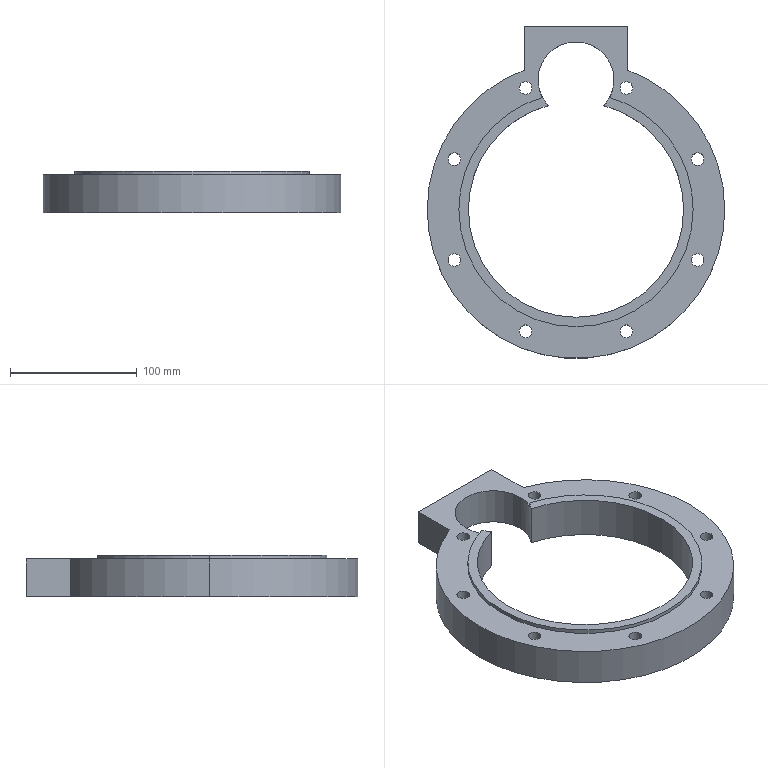Part | SolidWorks | features ICE 2, Cut 1, Extrusion 1, HoleWzd 1 | 1 solid | 34 faces | box 235 x 262.5 x 33 mm | volume 612977 mm3 | cylinder 28 | plane 6 | commonest cylinder face diameters 10 x16 60 x3 170 x3 185 x3 235 x3
STEP:
#1=CARTESIAN_POINT('',(26.584,88.598,30.));
#2=VERTEX_POINT('',#1);
#3=CARTESIAN_POINT('',(30.,102.5,30.));
#4=VERTEX_POINT('',#3);
#5=CARTESIAN_POINT('',(0.,102.5,30.));
#6=DIRECTION('',(0.,0.,1.));
#7=DIRECTION('',(1.,0.,0.));
#8=AXIS2_PLACEMENT_3D('',#5,#6,#7);
#9=CIRCLE('',#8,30.);
#10=EDGE_CURVE('',#2,#4,#9,.T.);
#11=ORIENTED_EDGE('',*,*,#10,.T.);
#12=CARTESIAN_POINT('',(30.,102.5,0.));
#13=VERTEX_POINT('',#12);
#14=CARTESIAN_POINT('',(30.,102.5,33.));
#15=DIRECTION('',(0.,0.,-1.));
#16=VECTOR('',#15,1000.);
#17=LINE('',#14,#16);
#18=EDGE_CURVE('',#4,#13,#17,.T.);
#19=ORIENTED_EDGE('',*,*,#18,.T.);
#20=CARTESIAN_POINT('',(22.,82.104,0.));
#21=VERTEX_POINT('',#20);
#22=CARTESIAN_POINT('',(0.,102.5,0.));
#23=DIRECTION('',(0.,0.,-1.));
#24=DIRECTION('',(-1.,0.,0.));
#25=AXIS2_PLACEMENT_3D('',#22,#23,#24);
#26=CIRCLE('',#25,30.);
#27=EDGE_CURVE('',#13,#21,#26,.T.);
#28=ORIENTED_EDGE('',*,*,#27,.T.);
#29=CARTESIAN_POINT('',(22.,82.104,33.));
#30=VERTEX_POINT('',#29);
#31=CARTESIAN_POINT('',(22.,82.104,16.5));
#32=DIRECTION('',(0.,0.,1.));
#33=VECTOR('',#32,1000.);
#34=LINE('',#31,#33);
#35=EDGE_CURVE('',#21,#30,#34,.T.);
#36=ORIENTED_EDGE('',*,*,#35,.T.);
#37=CARTESIAN_POINT('',(26.584,88.598,33.));
#38=VERTEX_POINT('',#37);
#39=CARTESIAN_POINT('',(0.,102.5,33.));
#40=DIRECTION('',(0.,0.,-1.));
#41=DIRECTION('',(-1.,0.,0.));
#42=AXIS2_PLACEMENT_3D('',#39,#40,#41);
#43=CIRCLE('',#42,30.);
#44=EDGE_CURVE('',#38,#30,#43,.T.);
#45=ORIENTED_EDGE('',*,*,#44,.F.);
#46=CARTESIAN_POINT('',(26.584,88.598,16.5));
#47=DIRECTION('',(0.,0.,1.));
#48=VECTOR('',#47,1000.);
#49=LINE('',#46,#48);
#50=EDGE_CURVE('',#2,#38,#49,.T.);
#51=ORIENTED_EDGE('',*,*,#50,.F.);
#52=EDGE_LOOP('',(#11,#19,#28,#36,#45,#51));
#53=FACE_OUTER_BOUND('',#52,.T.);
#54=CARTESIAN_POINT('',(0.,102.5,33.));
#55=DIRECTION('',(0.,0.,-1.));
#56=DIRECTION('',(-1.,0.,0.));
#57=AXIS2_PLACEMENT_3D('',#54,#55,#56);
#58=CYLINDRICAL_SURFACE('',#57,30.);
#59=ADVANCED_FACE('',(#53),#58,.F.);
#60=ORIENTED_EDGE('',*,*,#18,.F.);
#61=CARTESIAN_POINT('',(-30.,102.5,30.));
#62=VERTEX_POINT('',#61);
#63=CARTESIAN_POINT('',(0.,102.5,30.));
#64=DIRECTION('',(0.,0.,1.));
#65=DIRECTION('',(1.,0.,0.));
#66=AXIS2_PLACEMENT_3D('',#63,#64,#65);
#67=CIRCLE('',#66,30.);
#68=EDGE_CURVE('',#4,#62,#67,.T.);
#69=ORIENTED_EDGE('',*,*,#68,.T.);
#70=CARTESIAN_POINT('',(-30.,102.5,0.));
#71=VERTEX_POINT('',#70);
#72=CARTESIAN_POINT('',(-30.,102.5,33.));
#73=DIRECTION('',(0.,0.,-1.));
#74=VECTOR('',#73,1000.);
#75=LINE('',#72,#74);
#76=EDGE_CURVE('',#62,#71,#75,.T.);
#77=ORIENTED_EDGE('',*,*,#76,.T.);
#78=CARTESIAN_POINT('',(0.,102.5,0.));
#79=DIRECTION('',(0.,0.,-1.));
#80=DIRECTION('',(-1.,0.,0.));
#81=AXIS2_PLACEMENT_3D('',#78,#79,#80);
#82=CIRCLE('',#81,30.);
#83=EDGE_CURVE('',#71,#13,#82,.T.);
#84=ORIENTED_EDGE('',*,*,#83,.T.);
#85=EDGE_LOOP('',(#60,#69,#77,#84));
#86=FACE_OUTER_BOUND('',#85,.T.);
#87=CARTESIAN_POINT('',(0.,102.5,33.));
#88=DIRECTION('',(0.,0.,-1.));
#89=DIRECTION('',(-1.,0.,0.));
#90=AXIS2_PLACEMENT_3D('',#87,#88,#89);
#91=CYLINDRICAL_SURFACE('',#90,30.);
#92=ADVANCED_FACE('',(#86),#91,.F.);
#93=CARTESIAN_POINT('',(92.5,0.,33.));
#94=VERTEX_POINT('',#93);
#95=CARTESIAN_POINT('',(0.,0.,33.));
#96=DIRECTION('',(0.,0.,1.));
#97=DIRECTION('',(1.,0.,0.));
#98=AXIS2_PLACEMENT_3D('',#95,#96,#97);
#99=CIRCLE('',#98,92.5);
#100=EDGE_CURVE('',#94,#38,#99,.T.);
#101=ORIENTED_EDGE('',*,*,#100,.F.);
#102=CARTESIAN_POINT('',(92.5,0.,30.));
#103=VERTEX_POINT('',#102);
#104=CARTESIAN_POINT('',(92.5,0.,33.));
#105=DIRECTION('',(0.,0.,-1.));
#106=VECTOR('',#105,1000.);
#107=LINE('',#104,#106);
#108=EDGE_CURVE('',#94,#103,#107,.T.);
#109=ORIENTED_EDGE('',*,*,#108,.T.);
#110=CARTESIAN_POINT('',(0.,0.,30.));
#111=DIRECTION('',(0.,0.,1.));
#112=DIRECTION('',(1.,0.,0.));
#113=AXIS2_PLACEMENT_3D('',#110,#111,#112);
#114=CIRCLE('',#113,92.5);
#115=EDGE_CURVE('',#103,#2,#114,.T.);
#116=ORIENTED_EDGE('',*,*,#115,.T.);
#117=ORIENTED_EDGE('',*,*,#50,.T.);
#118=EDGE_LOOP('',(#101,#109,#116,#117));
#119=FACE_OUTER_BOUND('',#118,.T.);
#120=CARTESIAN_POINT('',(0.,0.,33.));
#121=DIRECTION('',(0.,0.,-1.));
#122=DIRECTION('',(-1.,0.,0.));
#123=AXIS2_PLACEMENT_3D('',#120,#121,#122);
#124=CYLINDRICAL_SURFACE('',#123,92.5);
#125=ADVANCED_FACE('',(#119),#124,.T.);
#126=ORIENTED_EDGE('',*,*,#108,.F.);
#127=CARTESIAN_POINT('',(-92.5,0.,33.));
#128=VERTEX_POINT('',#127);
#129=CARTESIAN_POINT('',(0.,0.,33.));
#130=DIRECTION('',(0.,0.,1.));
#131=DIRECTION('',(1.,0.,0.));
#132=AXIS2_PLACEMENT_3D('',#129,#130,#131);
#133=CIRCLE('',#132,92.5);
#134=EDGE_CURVE('',#128,#94,#133,.T.);
#135=ORIENTED_EDGE('',*,*,#134,.F.);
#136=CARTESIAN_POINT('',(-92.5,0.,30.));
#137=VERTEX_POINT('',#136);
#138=CARTESIAN_POINT('',(-92.5,0.,33.));
#139=DIRECTION('',(0.,0.,-1.));
#140=VECTOR('',#139,1000.);
#141=LINE('',#138,#140);
#142=EDGE_CURVE('',#128,#137,#141,.T.);
#143=ORIENTED_EDGE('',*,*,#142,.T.);
#144=CARTESIAN_POINT('',(0.,0.,30.));
#145=DIRECTION('',(0.,0.,1.));
#146=DIRECTION('',(1.,0.,0.));
#147=AXIS2_PLACEMENT_3D('',#144,#145,#146);
#148=CIRCLE('',#147,92.5);
#149=EDGE_CURVE('',#137,#103,#148,.T.);
#150=ORIENTED_EDGE('',*,*,#149,.T.);
#151=EDGE_LOOP('',(#126,#135,#143,#150));
#152=FACE_OUTER_BOUND('',#151,.T.);
#153=CARTESIAN_POINT('',(0.,0.,33.));
#154=DIRECTION('',(0.,0.,-1.));
#155=DIRECTION('',(-1.,0.,0.));
#156=AXIS2_PLACEMENT_3D('',#153,#154,#155);
#157=CYLINDRICAL_SURFACE('',#156,92.5);
#158=ADVANCED_FACE('',(#152),#157,.T.);
#159=CARTESIAN_POINT('',(44.799,96.083,30.));
#160=VERTEX_POINT('',#159);
#161=CARTESIAN_POINT('',(34.799,96.083,30.));
#162=VERTEX_POINT('',#161);
#163=CARTESIAN_POINT('',(39.799,96.083,30.));
#164=DIRECTION('',(0.,0.,-1.));
#165=DIRECTION('',(-1.,0.,0.));
#166=AXIS2_PLACEMENT_3D('',#163,#164,#165);
#167=CIRCLE('',#166,5.);
#168=EDGE_CURVE('',#160,#162,#167,.T.);
#169=ORIENTED_EDGE('',*,*,#168,.F.);
#170=CARTESIAN_POINT('',(44.799,96.083,0.));
#171=VERTEX_POINT('',#170);
#172=CARTESIAN_POINT('',(44.799,96.083,0.));
#173=DIRECTION('',(0.,0.,-1.));
#174=VECTOR('',#173,1000.);
#175=LINE('',#172,#174);
#176=EDGE_CURVE('',#160,#171,#175,.T.);
#177=ORIENTED_EDGE('',*,*,#176,.T.);
#178=CARTESIAN_POINT('',(34.799,96.083,0.));
#179=VERTEX_POINT('',#178);
#180=CARTESIAN_POINT('',(39.799,96.083,0.));
#181=DIRECTION('',(0.,0.,-1.));
#182=DIRECTION('',(-1.,0.,0.));
#183=AXIS2_PLACEMENT_3D('',#180,#181,#182);
#184=CIRCLE('',#183,5.);
#185=EDGE_CURVE('',#171,#179,#184,.T.);
#186=ORIENTED_EDGE('',*,*,#185,.T.);
#187=CARTESIAN_POINT('',(34.799,96.083,0.));
#188=DIRECTION('',(0.,0.,-1.));
#189=VECTOR('',#188,1000.);
#190=LINE('',#187,#189);
#191=EDGE_CURVE('',#162,#179,#190,.T.);
#192=ORIENTED_EDGE('',*,*,#191,.F.);
#193=EDGE_LOOP('',(#169,#177,#186,#192));
#194=FACE_OUTER_BOUND('',#193,.T.);
#195=CARTESIAN_POINT('',(39.799,96.083,0.));
#196=DIRECTION('',(0.,0.,-1.));
#197=DIRECTION('',(-1.,0.,0.));
#198=AXIS2_PLACEMENT_3D('',#195,#196,#197);
#199=CYLINDRICAL_SURFACE('',#198,5.);
#200=ADVANCED_FACE('',(#194),#199,.F.);
#201=CARTESIAN_POINT('',(-34.799,96.083,30.));
#202=VERTEX_POINT('',#201);
#203=CARTESIAN_POINT('',(-44.799,96.083,30.));
#204=VERTEX_POINT('',#203);
#205=CARTESIAN_POINT('',(-39.799,96.083,30.));
#206=DIRECTION('',(0.,0.,-1.));
#207=DIRECTION('',(-1.,0.,0.));
#208=AXIS2_PLACEMENT_3D('',#205,#206,#207);
#209=CIRCLE('',#208,5.);
#210=EDGE_CURVE('',#202,#204,#209,.T.);
#211=ORIENTED_EDGE('',*,*,#210,.F.);
#212=CARTESIAN_POINT('',(-34.799,96.083,0.));
#213=VERTEX_POINT('',#212);
#214=CARTESIAN_POINT('',(-34.799,96.083,0.));
#215=DIRECTION('',(0.,0.,-1.));
#216=VECTOR('',#215,1000.);
#217=LINE('',#214,#216);
#218=EDGE_CURVE('',#202,#213,#217,.T.);
#219=ORIENTED_EDGE('',*,*,#218,.T.);
#220=CARTESIAN_POINT('',(-44.799,96.083,0.));
#221=VERTEX_POINT('',#220);
#222=CARTESIAN_POINT('',(-39.799,96.083,0.));
#223=DIRECTION('',(0.,0.,-1.));
#224=DIRECTION('',(-1.,0.,0.));
#225=AXIS2_PLACEMENT_3D('',#222,#223,#224);
#226=CIRCLE('',#225,5.);
#227=EDGE_CURVE('',#213,#221,#226,.T.);
#228=ORIENTED_EDGE('',*,*,#227,.T.);
#229=CARTESIAN_POINT('',(-44.799,96.083,0.));
#230=DIRECTION('',(0.,0.,-1.));
#231=VECTOR('',#230,1000.);
#232=LINE('',#229,#231);
#233=EDGE_CURVE('',#204,#221,#232,.T.);
#234=ORIENTED_EDGE('',*,*,#233,.F.);
#235=EDGE_LOOP('',(#211,#219,#228,#234));
#236=FACE_OUTER_BOUND('',#235,.T.);
#237=CARTESIAN_POINT('',(-39.799,96.083,0.));
#238=DIRECTION('',(0.,0.,-1.));
#239=DIRECTION('',(-1.,0.,0.));
#240=AXIS2_PLACEMENT_3D('',#237,#238,#239);
#241=CYLINDRICAL_SURFACE('',#240,5.);
#242=ADVANCED_FACE('',(#236),#241,.F.);
#243=CARTESIAN_POINT('',(-91.083,39.799,30.));
#244=VERTEX_POINT('',#243);
#245=CARTESIAN_POINT('',(-101.083,39.799,30.));
#246=VERTEX_POINT('',#245);
#247=CARTESIAN_POINT('',(-96.083,39.799,30.));
#248=DIRECTION('',(0.,0.,-1.));
#249=DIRECTION('',(-1.,0.,0.));
#250=AXIS2_PLACEMENT_3D('',#247,#248,#249);
#251=CIRCLE('',#250,5.);
#252=EDGE_CURVE('',#244,#246,#251,.T.);
#253=ORIENTED_EDGE('',*,*,#252,.F.);
#254=CARTESIAN_POINT('',(-91.083,39.799,0.));
#255=VERTEX_POINT('',#254);
#256=CARTESIAN_POINT('',(-91.083,39.799,0.));
#257=DIRECTION('',(0.,0.,-1.));
#258=VECTOR('',#257,1000.);
#259=LINE('',#256,#258);
#260=EDGE_CURVE('',#244,#255,#259,.T.);
#261=ORIENTED_EDGE('',*,*,#260,.T.);
#262=CARTESIAN_POINT('',(-101.083,39.799,0.));
#263=VERTEX_POINT('',#262);
#264=CARTESIAN_POINT('',(-96.083,39.799,0.));
#265=DIRECTION('',(0.,0.,-1.));
#266=DIRECTION('',(-1.,0.,0.));
#267=AXIS2_PLACEMENT_3D('',#264,#265,#266);
#268=CIRCLE('',#267,5.);
#269=EDGE_CURVE('',#255,#263,#268,.T.);
#270=ORIENTED_EDGE('',*,*,#269,.T.);
#271=CARTESIAN_POINT('',(-101.083,39.799,0.));
#272=DIRECTION('',(0.,0.,-1.));
#273=VECTOR('',#272,1000.);
#274=LINE('',#271,#273);
#275=EDGE_CURVE('',#246,#263,#274,.T.);
#276=ORIENTED_EDGE('',*,*,#275,.F.);
#277=EDGE_LOOP('',(#253,#261,#270,#276));
#278=FACE_OUTER_BOUND('',#277,.T.);
#279=CARTESIAN_POINT('',(-96.083,39.799,0.));
#280=DIRECTION('',(0.,0.,-1.));
#281=DIRECTION('',(-1.,0.,0.));
#282=AXIS2_PLACEMENT_3D('',#279,#280,#281);
#283=CYLINDRICAL_SURFACE('',#282,5.);
#284=ADVANCED_FACE('',(#278),#283,.F.);
#285=CARTESIAN_POINT('',(-91.083,-39.799,30.));
#286=VERTEX_POINT('',#285);
#287=CARTESIAN_POINT('',(-101.083,-39.799,30.));
#288=VERTEX_POINT('',#287);
#289=CARTESIAN_POINT('',(-96.083,-39.799,30.));
#290=DIRECTION('',(0.,0.,-1.));
#291=DIRECTION('',(-1.,0.,0.));
#292=AXIS2_PLACEMENT_3D('',#289,#290,#291);
#293=CIRCLE('',#292,5.);
#294=EDGE_CURVE('',#286,#288,#293,.T.);
#295=ORIENTED_EDGE('',*,*,#294,.F.);
#296=CARTESIAN_POINT('',(-91.083,-39.799,0.));
#297=VERTEX_POINT('',#296);
#298=CARTESIAN_POINT('',(-91.083,-39.799,0.));
#299=DIRECTION('',(0.,0.,-1.));
#300=VECTOR('',#299,1000.);
#301=LINE('',#298,#300);
#302=EDGE_CURVE('',#286,#297,#301,.T.);
#303=ORIENTED_EDGE('',*,*,#302,.T.);
#304=CARTESIAN_POINT('',(-101.083,-39.799,0.));
#305=VERTEX_POINT('',#304);
#306=CARTESIAN_POINT('',(-96.083,-39.799,0.));
#307=DIRECTION('',(0.,0.,-1.));
#308=DIRECTION('',(-1.,0.,0.));
#309=AXIS2_PLACEMENT_3D('',#306,#307,#308);
#310=CIRCLE('',#309,5.);
#311=EDGE_CURVE('',#297,#305,#310,.T.);
#312=ORIENTED_EDGE('',*,*,#311,.T.);
#313=CARTESIAN_POINT('',(-101.083,-39.799,0.));
#314=DIRECTION('',(0.,0.,-1.));
#315=VECTOR('',#314,1000.);
#316=LINE('',#313,#315);
#317=EDGE_CURVE('',#288,#305,#316,.T.);
#318=ORIENTED_EDGE('',*,*,#317,.F.);
#319=EDGE_LOOP('',(#295,#303,#312,#318));
#320=FACE_OUTER_BOUND('',#319,.T.);
#321=CARTESIAN_POINT('',(-96.083,-39.799,0.));
#322=DIRECTION('',(0.,0.,-1.));
#323=DIRECTION('',(-1.,0.,0.));
#324=AXIS2_PLACEMENT_3D('',#321,#322,#323);
#325=CYLINDRICAL_SURFACE('',#324,5.);
#326=ADVANCED_FACE('',(#320),#325,.F.);
#327=CARTESIAN_POINT('',(-34.799,-96.083,30.));
#328=VERTEX_POINT('',#327);
#329=CARTESIAN_POINT('',(-44.799,-96.083,30.));
#330=VERTEX_POINT('',#329);
#331=CARTESIAN_POINT('',(-39.799,-96.083,30.));
#332=DIRECTION('',(0.,0.,-1.));
#333=DIRECTION('',(-1.,0.,0.));
#334=AXIS2_PLACEMENT_3D('',#331,#332,#333);
#335=CIRCLE('',#334,5.);
#336=EDGE_CURVE('',#328,#330,#335,.T.);
#337=ORIENTED_EDGE('',*,*,#336,.F.);
#338=CARTESIAN_POINT('',(-34.799,-96.083,0.));
#339=VERTEX_POINT('',#338);
#340=CARTESIAN_POINT('',(-34.799,-96.083,0.));
#341=DIRECTION('',(0.,0.,-1.));
#342=VECTOR('',#341,1000.);
#343=LINE('',#340,#342);
#344=EDGE_CURVE('',#328,#339,#343,.T.);
#345=ORIENTED_EDGE('',*,*,#344,.T.);
#346=CARTESIAN_POINT('',(-44.799,-96.083,0.));
#347=VERTEX_POINT('',#346);
#348=CARTESIAN_POINT('',(-39.799,-96.083,0.));
#349=DIRECTION('',(0.,0.,-1.));
#350=DIRECTION('',(-1.,0.,0.));
#351=AXIS2_PLACEMENT_3D('',#348,#349,#350);
#352=CIRCLE('',#351,5.);
#353=EDGE_CURVE('',#339,#347,#352,.T.);
#354=ORIENTED_EDGE('',*,*,#353,.T.);
#355=CARTESIAN_POINT('',(-44.799,-96.083,0.));
#356=DIRECTION('',(0.,0.,-1.));
#357=VECTOR('',#356,1000.);
#358=LINE('',#355,#357);
#359=EDGE_CURVE('',#330,#347,#358,.T.);
#360=ORIENTED_EDGE('',*,*,#359,.F.);
#361=EDGE_LOOP('',(#337,#345,#354,#360));
#362=FACE_OUTER_BOUND('',#361,.T.);
#363=CARTESIAN_POINT('',(-39.799,-96.083,0.));
#364=DIRECTION('',(0.,0.,-1.));
#365=DIRECTION('',(-1.,0.,0.));
#366=AXIS2_PLACEMENT_3D('',#363,#364,#365);
#367=CYLINDRICAL_SURFACE('',#366,5.);
#368=ADVANCED_FACE('',(#362),#367,.F.);
#369=CARTESIAN_POINT('',(44.799,-96.083,30.));
#370=VERTEX_POINT('',#369);
#371=CARTESIAN_POINT('',(34.799,-96.083,30.));
#372=VERTEX_POINT('',#371);
#373=CARTESIAN_POINT('',(39.799,-96.083,30.));
#374=DIRECTION('',(0.,0.,-1.));
#375=DIRECTION('',(-1.,0.,0.));
#376=AXIS2_PLACEMENT_3D('',#373,#374,#375);
#377=CIRCLE('',#376,5.);
#378=EDGE_CURVE('',#370,#372,#377,.T.);
#379=ORIENTED_EDGE('',*,*,#378,.F.);
#380=CARTESIAN_POINT('',(44.799,-96.083,0.));
#381=VERTEX_POINT('',#380);
#382=CARTESIAN_POINT('',(44.799,-96.083,0.));
#383=DIRECTION('',(0.,0.,-1.));
#384=VECTOR('',#383,1000.);
#385=LINE('',#382,#384);
#386=EDGE_CURVE('',#370,#381,#385,.T.);
#387=ORIENTED_EDGE('',*,*,#386,.T.);
#388=CARTESIAN_POINT('',(34.799,-96.083,0.));
#389=VERTEX_POINT('',#388);
#390=CARTESIAN_POINT('',(39.799,-96.083,0.));
#391=DIRECTION('',(0.,0.,-1.));
#392=DIRECTION('',(-1.,0.,0.));
#393=AXIS2_PLACEMENT_3D('',#390,#391,#392);
#394=CIRCLE('',#393,5.);
#395=EDGE_CURVE('',#381,#389,#394,.T.);
#396=ORIENTED_EDGE('',*,*,#395,.T.);
#397=CARTESIAN_POINT('',(34.799,-96.083,0.));
#398=DIRECTION('',(0.,0.,-1.));
#399=VECTOR('',#398,1000.);
#400=LINE('',#397,#399);
#401=EDGE_CURVE('',#372,#389,#400,.T.);
#402=ORIENTED_EDGE('',*,*,#401,.F.);
#403=EDGE_LOOP('',(#379,#387,#396,#402));
#404=FACE_OUTER_BOUND('',#403,.T.);
#405=CARTESIAN_POINT('',(39.799,-96.083,0.));
#406=DIRECTION('',(0.,0.,-1.));
#407=DIRECTION('',(-1.,0.,0.));
#408=AXIS2_PLACEMENT_3D('',#405,#406,#407);
#409=CYLINDRICAL_SURFACE('',#408,5.);
#410=ADVANCED_FACE('',(#404),#409,.F.);
#411=CARTESIAN_POINT('',(101.083,-39.799,30.));
#412=VERTEX_POINT('',#411);
#413=CARTESIAN_POINT('',(91.083,-39.799,30.));
#414=VERTEX_POINT('',#413);
#415=CARTESIAN_POINT('',(96.083,-39.799,30.));
#416=DIRECTION('',(0.,0.,-1.));
#417=DIRECTION('',(-1.,0.,0.));
#418=AXIS2_PLACEMENT_3D('',#415,#416,#417);
#419=CIRCLE('',#418,5.);
#420=EDGE_CURVE('',#412,#414,#419,.T.);
#421=ORIENTED_EDGE('',*,*,#420,.F.);
#422=CARTESIAN_POINT('',(101.083,-39.799,0.));
#423=VERTEX_POINT('',#422);
#424=CARTESIAN_POINT('',(101.083,-39.799,0.));
#425=DIRECTION('',(0.,0.,-1.));
#426=VECTOR('',#425,1000.);
#427=LINE('',#424,#426);
#428=EDGE_CURVE('',#412,#423,#427,.T.);
#429=ORIENTED_EDGE('',*,*,#428,.T.);
#430=CARTESIAN_POINT('',(91.083,-39.799,0.));
#431=VERTEX_POINT('',#430);
#432=CARTESIAN_POINT('',(96.083,-39.799,0.));
#433=DIRECTION('',(0.,0.,-1.));
#434=DIRECTION('',(-1.,0.,0.));
#435=AXIS2_PLACEMENT_3D('',#432,#433,#434);
#436=CIRCLE('',#435,5.);
#437=EDGE_CURVE('',#423,#431,#436,.T.);
#438=ORIENTED_EDGE('',*,*,#437,.T.);
#439=CARTESIAN_POINT('',(91.083,-39.799,0.));
#440=DIRECTION('',(0.,0.,-1.));
#441=VECTOR('',#440,1000.);
#442=LINE('',#439,#441);
#443=EDGE_CURVE('',#414,#431,#442,.T.);
#444=ORIENTED_EDGE('',*,*,#443,.F.);
#445=EDGE_LOOP('',(#421,#429,#438,#444));
#446=FACE_OUTER_BOUND('',#445,.T.);
#447=CARTESIAN_POINT('',(96.083,-39.799,0.));
#448=DIRECTION('',(0.,0.,-1.));
#449=DIRECTION('',(-1.,0.,0.));
#450=AXIS2_PLACEMENT_3D('',#447,#448,#449);
#451=CYLINDRICAL_SURFACE('',#450,5.);
#452=ADVANCED_FACE('',(#446),#451,.F.);
#453=CARTESIAN_POINT('',(101.083,39.799,30.));
#454=VERTEX_POINT('',#453);
#455=CARTESIAN_POINT('',(91.083,39.799,30.));
#456=VERTEX_POINT('',#455);
#457=CARTESIAN_POINT('',(96.083,39.799,30.));
#458=DIRECTION('',(0.,0.,-1.));
#459=DIRECTION('',(-1.,0.,0.));
#460=AXIS2_PLACEMENT_3D('',#457,#458,#459);
#461=CIRCLE('',#460,5.);
#462=EDGE_CURVE('',#454,#456,#461,.T.);
#463=ORIENTED_EDGE('',*,*,#462,.F.);
#464=CARTESIAN_POINT('',(101.083,39.799,0.));
#465=VERTEX_POINT('',#464);
#466=CARTESIAN_POINT('',(101.083,39.799,0.));
#467=DIRECTION('',(0.,0.,-1.));
#468=VECTOR('',#467,1000.);
#469=LINE('',#466,#468);
#470=EDGE_CURVE('',#454,#465,#469,.T.);
#471=ORIENTED_EDGE('',*,*,#470,.T.);
#472=CARTESIAN_POINT('',(91.083,39.799,0.));
#473=VERTEX_POINT('',#472);
#474=CARTESIAN_POINT('',(96.083,39.799,0.));
#475=DIRECTION('',(0.,0.,-1.));
#476=DIRECTION('',(-1.,0.,0.));
#477=AXIS2_PLACEMENT_3D('',#474,#475,#476);
#478=CIRCLE('',#477,5.);
#479=EDGE_CURVE('',#465,#473,#478,.T.);
#480=ORIENTED_EDGE('',*,*,#479,.T.);
#481=CARTESIAN_POINT('',(91.083,39.799,0.));
#482=DIRECTION('',(0.,0.,-1.));
#483=VECTOR('',#482,1000.);
#484=LINE('',#481,#483);
#485=EDGE_CURVE('',#456,#473,#484,.T.);
#486=ORIENTED_EDGE('',*,*,#485,.F.);
#487=EDGE_LOOP('',(#463,#471,#480,#486));
#488=FACE_OUTER_BOUND('',#487,.T.);
#489=CARTESIAN_POINT('',(96.083,39.799,0.));
#490=DIRECTION('',(0.,0.,-1.));
#491=DIRECTION('',(-1.,0.,0.));
#492=AXIS2_PLACEMENT_3D('',#489,#490,#491);
#493=CYLINDRICAL_SURFACE('',#492,5.);
#494=ADVANCED_FACE('',(#488),#493,.F.);
#495=CARTESIAN_POINT('',(-85.,0.,33.));
#496=VERTEX_POINT('',#495);
#497=CARTESIAN_POINT('',(85.,0.,33.));
#498=VERTEX_POINT('',#497);
#499=CARTESIAN_POINT('',(0.,0.,33.));
#500=DIRECTION('',(0.,0.,1.));
#501=DIRECTION('',(1.,0.,0.));
#502=AXIS2_PLACEMENT_3D('',#499,#500,#501);
#503=CIRCLE('',#502,85.);
#504=EDGE_CURVE('',#496,#498,#503,.T.);
#505=ORIENTED_EDGE('',*,*,#504,.T.);
#506=CARTESIAN_POINT('',(85.,0.,0.));
#507=VERTEX_POINT('',#506);
#508=CARTESIAN_POINT('',(85.,0.,30.));
#509=DIRECTION('',(0.,0.,-1.));
#510=VECTOR('',#509,1000.);
#511=LINE('',#508,#510);
#512=EDGE_CURVE('',#498,#507,#511,.T.);
#513=ORIENTED_EDGE('',*,*,#512,.T.);
#514=CARTESIAN_POINT('',(-85.,0.,0.));
#515=VERTEX_POINT('',#514);
#516=CARTESIAN_POINT('',(0.,0.,0.));
#517=DIRECTION('',(0.,0.,1.));
#518=DIRECTION('',(1.,0.,0.));
#519=AXIS2_PLACEMENT_3D('',#516,#517,#518);
#520=CIRCLE('',#519,85.);
#521=EDGE_CURVE('',#515,#507,#520,.T.);
#522=ORIENTED_EDGE('',*,*,#521,.F.);
#523=CARTESIAN_POINT('',(-85.,0.,30.));
#524=DIRECTION('',(0.,0.,-1.));
#525=VECTOR('',#524,1000.);
#526=LINE('',#523,#525);
#527=EDGE_CURVE('',#496,#515,#526,.T.);
#528=ORIENTED_EDGE('',*,*,#527,.F.);
#529=EDGE_LOOP('',(#505,#513,#522,#528));
#530=FACE_OUTER_BOUND('',#529,.T.);
#531=CARTESIAN_POINT('',(0.,0.,30.));
#532=DIRECTION('',(0.,0.,-1.));
#533=DIRECTION('',(-1.,0.,0.));
#534=AXIS2_PLACEMENT_3D('',#531,#532,#533);
#535=CYLINDRICAL_SURFACE('',#534,85.);
#536=ADVANCED_FACE('',(#530),#535,.F.);
#537=CARTESIAN_POINT('',(-22.,82.104,33.));
#538=VERTEX_POINT('',#537);
#539=CARTESIAN_POINT('',(0.,0.,33.));
#540=DIRECTION('',(0.,0.,1.));
#541=DIRECTION('',(1.,0.,0.));
#542=AXIS2_PLACEMENT_3D('',#539,#540,#541);
#543=CIRCLE('',#542,85.);
#544=EDGE_CURVE('',#538,#496,#543,.T.);
#545=ORIENTED_EDGE('',*,*,#544,.T.);
#546=ORIENTED_EDGE('',*,*,#527,.T.);
#547=CARTESIAN_POINT('',(-22.,82.104,0.));
#548=VERTEX_POINT('',#547);
#549=CARTESIAN_POINT('',(0.,0.,0.));
#550=DIRECTION('',(0.,0.,1.));
#551=DIRECTION('',(1.,0.,0.));
#552=AXIS2_PLACEMENT_3D('',#549,#550,#551);
#553=CIRCLE('',#552,85.);
#554=EDGE_CURVE('',#548,#515,#553,.T.);
#555=ORIENTED_EDGE('',*,*,#554,.F.);
#556=CARTESIAN_POINT('',(-22.,82.104,16.5));
#557=DIRECTION('',(0.,0.,-1.));
#558=VECTOR('',#557,1000.);
#559=LINE('',#556,#558);
#560=EDGE_CURVE('',#538,#548,#559,.T.);
#561=ORIENTED_EDGE('',*,*,#560,.F.);
#562=EDGE_LOOP('',(#545,#546,#555,#561));
#563=FACE_OUTER_BOUND('',#562,.T.);
#564=CARTESIAN_POINT('',(0.,0.,30.));
#565=DIRECTION('',(0.,0.,-1.));
#566=DIRECTION('',(-1.,0.,0.));
#567=AXIS2_PLACEMENT_3D('',#564,#565,#566);
#568=CYLINDRICAL_SURFACE('',#567,85.);
#569=ADVANCED_FACE('',(#563),#568,.F.);
#570=CARTESIAN_POINT('',(117.5,0.,30.));
#571=VERTEX_POINT('',#570);
#572=CARTESIAN_POINT('',(41.,110.115,30.));
#573=VERTEX_POINT('',#572);
#574=CARTESIAN_POINT('',(0.,0.,30.));
#575=DIRECTION('',(0.,0.,1.));
#576=DIRECTION('',(1.,0.,0.));
#577=AXIS2_PLACEMENT_3D('',#574,#575,#576);
#578=CIRCLE('',#577,117.5);
#579=EDGE_CURVE('',#571,#573,#578,.T.);
#580=ORIENTED_EDGE('',*,*,#579,.F.);
#581=CARTESIAN_POINT('',(117.5,0.,0.));
#582=VERTEX_POINT('',#581);
#583=CARTESIAN_POINT('',(117.5,0.,30.));
#584=DIRECTION('',(0.,0.,-1.));
#585=VECTOR('',#584,1000.);
#586=LINE('',#583,#585);
#587=EDGE_CURVE('',#571,#582,#586,.T.);
#588=ORIENTED_EDGE('',*,*,#587,.T.);
#589=CARTESIAN_POINT('',(41.,110.115,0.));
#590=VERTEX_POINT('',#589);
#591=CARTESIAN_POINT('',(0.,0.,0.));
#592=DIRECTION('',(0.,0.,1.));
#593=DIRECTION('',(1.,0.,0.));
#594=AXIS2_PLACEMENT_3D('',#591,#592,#593);
#595=CIRCLE('',#594,117.5);
#596=EDGE_CURVE('',#582,#590,#595,.T.);
#597=ORIENTED_EDGE('',*,*,#596,.T.);
#598=CARTESIAN_POINT('',(41.,110.115,30.));
#599=DIRECTION('',(0.,0.,1.));
#600=VECTOR('',#599,1000.);
#601=LINE('',#598,#600);
#602=EDGE_CURVE('',#590,#573,#601,.T.);
#603=ORIENTED_EDGE('',*,*,#602,.T.);
#604=EDGE_LOOP('',(#580,#588,#597,#603));
#605=FACE_OUTER_BOUND('',#604,.T.);
#606=CARTESIAN_POINT('',(0.,0.,30.));
#607=DIRECTION('',(0.,0.,-1.));
#608=DIRECTION('',(-1.,0.,0.));
#609=AXIS2_PLACEMENT_3D('',#606,#607,#608);
#610=CYLINDRICAL_SURFACE('',#609,117.5);
#611=ADVANCED_FACE('',(#605),#610,.T.);
#612=ORIENTED_EDGE('',*,*,#587,.F.);
#613=CARTESIAN_POINT('',(-117.5,0.,30.));
#614=VERTEX_POINT('',#613);
#615=CARTESIAN_POINT('',(0.,0.,30.));
#616=DIRECTION('',(0.,0.,1.));
#617=DIRECTION('',(1.,0.,0.));
#618=AXIS2_PLACEMENT_3D('',#615,#616,#617);
#619=CIRCLE('',#618,117.5);
#620=EDGE_CURVE('',#614,#571,#619,.T.);
#621=ORIENTED_EDGE('',*,*,#620,.F.);
#622=CARTESIAN_POINT('',(-117.5,0.,0.));
#623=VERTEX_POINT('',#622);
#624=CARTESIAN_POINT('',(-117.5,0.,30.));
#625=DIRECTION('',(0.,0.,-1.));
#626=VECTOR('',#625,1000.);
#627=LINE('',#624,#626);
#628=EDGE_CURVE('',#614,#623,#627,.T.);
#629=ORIENTED_EDGE('',*,*,#628,.T.);
#630=CARTESIAN_POINT('',(0.,0.,0.));
#631=DIRECTION('',(0.,0.,1.));
#632=DIRECTION('',(1.,0.,0.));
#633=AXIS2_PLACEMENT_3D('',#630,#631,#632);
#634=CIRCLE('',#633,117.5);
#635=EDGE_CURVE('',#623,#582,#634,.T.);
#636=ORIENTED_EDGE('',*,*,#635,.T.);
#637=EDGE_LOOP('',(#612,#621,#629,#636));
#638=FACE_OUTER_BOUND('',#637,.T.);
#639=CARTESIAN_POINT('',(0.,0.,30.));
#640=DIRECTION('',(0.,0.,-1.));
#641=DIRECTION('',(-1.,0.,0.));
#642=AXIS2_PLACEMENT_3D('',#639,#640,#641);
#643=CYLINDRICAL_SURFACE('',#642,117.5);
#644=ADVANCED_FACE('',(#638),#643,.T.);
#645=ORIENTED_EDGE('',*,*,#10,.F.);
#646=ORIENTED_EDGE('',*,*,#115,.F.);
#647=ORIENTED_EDGE('',*,*,#149,.F.);
#648=CARTESIAN_POINT('',(-26.584,88.598,30.));
#649=VERTEX_POINT('',#648);
#650=CARTESIAN_POINT('',(0.,0.,30.));
#651=DIRECTION('',(0.,0.,1.));
#652=DIRECTION('',(1.,0.,0.));
#653=AXIS2_PLACEMENT_3D('',#650,#651,#652);
#654=CIRCLE('',#653,92.5);
#655=EDGE_CURVE('',#649,#137,#654,.T.);
#656=ORIENTED_EDGE('',*,*,#655,.F.);
#657=CARTESIAN_POINT('',(0.,102.5,30.));
#658=DIRECTION('',(0.,0.,1.));
#659=DIRECTION('',(1.,0.,0.));
#660=AXIS2_PLACEMENT_3D('',#657,#658,#659);
#661=CIRCLE('',#660,30.);
#662=EDGE_CURVE('',#62,#649,#661,.T.);
#663=ORIENTED_EDGE('',*,*,#662,.F.);
#664=ORIENTED_EDGE('',*,*,#68,.F.);
#665=EDGE_LOOP('',(#645,#646,#647,#656,#663,#664));
#666=FACE_BOUND('',#665,.T.);
#667=CARTESIAN_POINT('',(39.799,-96.083,30.));
#668=DIRECTION('',(0.,0.,-1.));
#669=DIRECTION('',(-1.,0.,0.));
#670=AXIS2_PLACEMENT_3D('',#667,#668,#669);
#671=CIRCLE('',#670,5.);
#672=EDGE_CURVE('',#372,#370,#671,.T.);
#673=ORIENTED_EDGE('',*,*,#672,.T.);
#674=ORIENTED_EDGE('',*,*,#378,.T.);
#675=EDGE_LOOP('',(#673,#674));
#676=FACE_BOUND('',#675,.T.);
#677=CARTESIAN_POINT('',(96.083,-39.799,30.));
#678=DIRECTION('',(0.,0.,-1.));
#679=DIRECTION('',(-1.,0.,0.));
#680=AXIS2_PLACEMENT_3D('',#677,#678,#679);
#681=CIRCLE('',#680,5.);
#682=EDGE_CURVE('',#414,#412,#681,.T.);
#683=ORIENTED_EDGE('',*,*,#682,.T.);
#684=ORIENTED_EDGE('',*,*,#420,.T.);
#685=EDGE_LOOP('',(#683,#684));
#686=FACE_BOUND('',#685,.T.);
#687=CARTESIAN_POINT('',(96.083,39.799,30.));
#688=DIRECTION('',(0.,0.,-1.));
#689=DIRECTION('',(-1.,0.,0.));
#690=AXIS2_PLACEMENT_3D('',#687,#688,#689);
#691=CIRCLE('',#690,5.);
#692=EDGE_CURVE('',#456,#454,#691,.T.);
#693=ORIENTED_EDGE('',*,*,#692,.T.);
#694=ORIENTED_EDGE('',*,*,#462,.T.);
#695=EDGE_LOOP('',(#693,#694));
#696=FACE_BOUND('',#695,.T.);
#697=CARTESIAN_POINT('',(-41.,110.115,30.));
#698=VERTEX_POINT('',#697);
#699=CARTESIAN_POINT('',(0.,0.,30.));
#700=DIRECTION('',(0.,0.,1.));
#701=DIRECTION('',(1.,0.,0.));
#702=AXIS2_PLACEMENT_3D('',#699,#700,#701);
#703=CIRCLE('',#702,117.5);
#704=EDGE_CURVE('',#698,#614,#703,.T.);
#705=ORIENTED_EDGE('',*,*,#704,.T.);
#706=ORIENTED_EDGE('',*,*,#620,.T.);
#707=ORIENTED_EDGE('',*,*,#579,.T.);
#708=CARTESIAN_POINT('',(41.,145.,30.));
#709=VERTEX_POINT('',#708);
#710=CARTESIAN_POINT('',(41.,85.,30.));
#711=DIRECTION('',(0.,1.,0.));
#712=VECTOR('',#711,1000.);
#713=LINE('',#710,#712);
#714=EDGE_CURVE('',#573,#709,#713,.T.);
#715=ORIENTED_EDGE('',*,*,#714,.T.);
#716=CARTESIAN_POINT('',(-41.,145.,30.));
#717=VERTEX_POINT('',#716);
#718=CARTESIAN_POINT('',(-41.,145.,30.));
#719=DIRECTION('',(-1.,0.,0.));
#720=VECTOR('',#719,1000.);
#721=LINE('',#718,#720);
#722=EDGE_CURVE('',#709,#717,#721,.T.);
#723=ORIENTED_EDGE('',*,*,#722,.T.);
#724=CARTESIAN_POINT('',(-41.,85.,30.));
#725=DIRECTION('',(0.,-1.,0.));
#726=VECTOR('',#725,1000.);
#727=LINE('',#724,#726);
#728=EDGE_CURVE('',#717,#698,#727,.T.);
#729=ORIENTED_EDGE('',*,*,#728,.T.);
#730=EDGE_LOOP('',(#705,#706,#707,#715,#723,#729));
#731=FACE_OUTER_BOUND('',#730,.T.);
#732=CARTESIAN_POINT('',(-39.799,-96.083,30.));
#733=DIRECTION('',(0.,0.,-1.));
#734=DIRECTION('',(-1.,0.,0.));
#735=AXIS2_PLACEMENT_3D('',#732,#733,#734);
#736=CIRCLE('',#735,5.);
#737=EDGE_CURVE('',#330,#328,#736,.T.);
#738=ORIENTED_EDGE('',*,*,#737,.T.);
#739=ORIENTED_EDGE('',*,*,#336,.T.);
#740=EDGE_LOOP('',(#738,#739));
#741=FACE_BOUND('',#740,.T.);
#742=CARTESIAN_POINT('',(-96.083,-39.799,30.));
#743=DIRECTION('',(0.,0.,-1.));
#744=DIRECTION('',(-1.,0.,0.));
#745=AXIS2_PLACEMENT_3D('',#742,#743,#744);
#746=CIRCLE('',#745,5.);
#747=EDGE_CURVE('',#288,#286,#746,.T.);
#748=ORIENTED_EDGE('',*,*,#747,.T.);
#749=ORIENTED_EDGE('',*,*,#294,.T.);
#750=EDGE_LOOP('',(#748,#749));
#751=FACE_BOUND('',#750,.T.);
#752=CARTESIAN_POINT('',(-96.083,39.799,30.));
#753=DIRECTION('',(0.,0.,-1.));
#754=DIRECTION('',(-1.,0.,0.));
#755=AXIS2_PLACEMENT_3D('',#752,#753,#754);
#756=CIRCLE('',#755,5.);
#757=EDGE_CURVE('',#246,#244,#756,.T.);
#758=ORIENTED_EDGE('',*,*,#757,.T.);
#759=ORIENTED_EDGE('',*,*,#252,.T.);
#760=EDGE_LOOP('',(#758,#759));
#761=FACE_BOUND('',#760,.T.);
#762=CARTESIAN_POINT('',(-39.799,96.083,30.));
#763=DIRECTION('',(0.,0.,-1.));
#764=DIRECTION('',(-1.,0.,0.));
#765=AXIS2_PLACEMENT_3D('',#762,#763,#764);
#766=CIRCLE('',#765,5.);
#767=EDGE_CURVE('',#204,#202,#766,.T.);
#768=ORIENTED_EDGE('',*,*,#767,.T.);
#769=ORIENTED_EDGE('',*,*,#210,.T.);
#770=EDGE_LOOP('',(#768,#769));
#771=FACE_BOUND('',#770,.T.);
#772=CARTESIAN_POINT('',(39.799,96.083,30.));
#773=DIRECTION('',(0.,0.,-1.));
#774=DIRECTION('',(-1.,0.,0.));
#775=AXIS2_PLACEMENT_3D('',#772,#773,#774);
#776=CIRCLE('',#775,5.);
#777=EDGE_CURVE('',#162,#160,#776,.T.);
#778=ORIENTED_EDGE('',*,*,#777,.T.);
#779=ORIENTED_EDGE('',*,*,#168,.T.);
#780=EDGE_LOOP('',(#778,#779));
#781=FACE_BOUND('',#780,.T.);
#782=CARTESIAN_POINT('',(0.,0.,30.));
#783=DIRECTION('',(0.,0.,1.));
#784=DIRECTION('',(1.,0.,0.));
#785=AXIS2_PLACEMENT_3D('',#782,#783,#784);
#786=PLANE('',#785);
#787=ADVANCED_FACE('',(#666,#676,#686,#696,#731,#741,#751,#761,#771,#781),#786,.T.);
#788=CARTESIAN_POINT('',(39.799,96.083,0.));
#789=DIRECTION('',(0.,0.,-1.));
#790=DIRECTION('',(-1.,0.,0.));
#791=AXIS2_PLACEMENT_3D('',#788,#789,#790);
#792=CIRCLE('',#791,5.);
#793=EDGE_CURVE('',#179,#171,#792,.T.);
#794=ORIENTED_EDGE('',*,*,#793,.F.);
#795=ORIENTED_EDGE('',*,*,#185,.F.);
#796=EDGE_LOOP('',(#794,#795));
#797=FACE_BOUND('',#796,.T.);
#798=CARTESIAN_POINT('',(-39.799,96.083,0.));
#799=DIRECTION('',(0.,0.,-1.));
#800=DIRECTION('',(-1.,0.,0.));
#801=AXIS2_PLACEMENT_3D('',#798,#799,#800);
#802=CIRCLE('',#801,5.);
#803=EDGE_CURVE('',#221,#213,#802,.T.);
#804=ORIENTED_EDGE('',*,*,#803,.F.);
#805=ORIENTED_EDGE('',*,*,#227,.F.);
#806=EDGE_LOOP('',(#804,#805));
#807=FACE_BOUND('',#806,.T.);
#808=CARTESIAN_POINT('',(-96.083,39.799,0.));
#809=DIRECTION('',(0.,0.,-1.));
#810=DIRECTION('',(-1.,0.,0.));
#811=AXIS2_PLACEMENT_3D('',#808,#809,#810);
#812=CIRCLE('',#811,5.);
#813=EDGE_CURVE('',#263,#255,#812,.T.);
#814=ORIENTED_EDGE('',*,*,#813,.F.);
#815=ORIENTED_EDGE('',*,*,#269,.F.);
#816=EDGE_LOOP('',(#814,#815));
#817=FACE_BOUND('',#816,.T.);
#818=CARTESIAN_POINT('',(-96.083,-39.799,0.));
#819=DIRECTION('',(0.,0.,-1.));
#820=DIRECTION('',(-1.,0.,0.));
#821=AXIS2_PLACEMENT_3D('',#818,#819,#820);
#822=CIRCLE('',#821,5.);
#823=EDGE_CURVE('',#305,#297,#822,.T.);
#824=ORIENTED_EDGE('',*,*,#823,.F.);
#825=ORIENTED_EDGE('',*,*,#311,.F.);
#826=EDGE_LOOP('',(#824,#825));
#827=FACE_BOUND('',#826,.T.);
#828=CARTESIAN_POINT('',(-39.799,-96.083,0.));
#829=DIRECTION('',(0.,0.,-1.));
#830=DIRECTION('',(-1.,0.,0.));
#831=AXIS2_PLACEMENT_3D('',#828,#829,#830);
#832=CIRCLE('',#831,5.);
#833=EDGE_CURVE('',#347,#339,#832,.T.);
#834=ORIENTED_EDGE('',*,*,#833,.F.);
#835=ORIENTED_EDGE('',*,*,#353,.F.);
#836=EDGE_LOOP('',(#834,#835));
#837=FACE_BOUND('',#836,.T.);
#838=CARTESIAN_POINT('',(39.799,-96.083,0.));
#839=DIRECTION('',(0.,0.,-1.));
#840=DIRECTION('',(-1.,0.,0.));
#841=AXIS2_PLACEMENT_3D('',#838,#839,#840);
#842=CIRCLE('',#841,5.);
#843=EDGE_CURVE('',#389,#381,#842,.T.);
#844=ORIENTED_EDGE('',*,*,#843,.F.);
#845=ORIENTED_EDGE('',*,*,#395,.F.);
#846=EDGE_LOOP('',(#844,#845));
#847=FACE_BOUND('',#846,.T.);
#848=CARTESIAN_POINT('',(96.083,39.799,0.));
#849=DIRECTION('',(0.,0.,-1.));
#850=DIRECTION('',(-1.,0.,0.));
#851=AXIS2_PLACEMENT_3D('',#848,#849,#850);
#852=CIRCLE('',#851,5.);
#853=EDGE_CURVE('',#473,#465,#852,.T.);
#854=ORIENTED_EDGE('',*,*,#853,.F.);
#855=ORIENTED_EDGE('',*,*,#479,.F.);
#856=EDGE_LOOP('',(#854,#855));
#857=FACE_BOUND('',#856,.T.);
#858=CARTESIAN_POINT('',(41.,145.,0.));
#859=VERTEX_POINT('',#858);
#860=CARTESIAN_POINT('',(41.,85.,0.));
#861=DIRECTION('',(0.,1.,0.));
#862=VECTOR('',#861,1000.);
#863=LINE('',#860,#862);
#864=EDGE_CURVE('',#590,#859,#863,.T.);
#865=ORIENTED_EDGE('',*,*,#864,.F.);
#866=ORIENTED_EDGE('',*,*,#596,.F.);
#867=ORIENTED_EDGE('',*,*,#635,.F.);
#868=CARTESIAN_POINT('',(-41.,110.115,0.));
#869=VERTEX_POINT('',#868);
#870=CARTESIAN_POINT('',(0.,0.,0.));
#871=DIRECTION('',(0.,0.,1.));
#872=DIRECTION('',(1.,0.,0.));
#873=AXIS2_PLACEMENT_3D('',#870,#871,#872);
#874=CIRCLE('',#873,117.5);
#875=EDGE_CURVE('',#869,#623,#874,.T.);
#876=ORIENTED_EDGE('',*,*,#875,.F.);
#877=CARTESIAN_POINT('',(-41.,145.,0.));
#878=VERTEX_POINT('',#877);
#879=CARTESIAN_POINT('',(-41.,85.,0.));
#880=DIRECTION('',(0.,-1.,0.));
#881=VECTOR('',#880,1000.);
#882=LINE('',#879,#881);
#883=EDGE_CURVE('',#878,#869,#882,.T.);
#884=ORIENTED_EDGE('',*,*,#883,.F.);
#885=CARTESIAN_POINT('',(-41.,145.,0.));
#886=DIRECTION('',(-1.,0.,0.));
#887=VECTOR('',#886,1000.);
#888=LINE('',#885,#887);
#889=EDGE_CURVE('',#859,#878,#888,.T.);
#890=ORIENTED_EDGE('',*,*,#889,.F.);
#891=EDGE_LOOP('',(#865,#866,#867,#876,#884,#890));
#892=FACE_OUTER_BOUND('',#891,.T.);
#893=ORIENTED_EDGE('',*,*,#554,.T.);
#894=ORIENTED_EDGE('',*,*,#521,.T.);
#895=CARTESIAN_POINT('',(0.,0.,0.));
#896=DIRECTION('',(0.,0.,1.));
#897=DIRECTION('',(1.,0.,0.));
#898=AXIS2_PLACEMENT_3D('',#895,#896,#897);
#899=CIRCLE('',#898,85.);
#900=EDGE_CURVE('',#507,#21,#899,.T.);
#901=ORIENTED_EDGE('',*,*,#900,.T.);
#902=ORIENTED_EDGE('',*,*,#27,.F.);
#903=ORIENTED_EDGE('',*,*,#83,.F.);
#904=CARTESIAN_POINT('',(0.,102.5,0.));
#905=DIRECTION('',(0.,0.,-1.));
#906=DIRECTION('',(-1.,0.,0.));
#907=AXIS2_PLACEMENT_3D('',#904,#905,#906);
#908=CIRCLE('',#907,30.);
#909=EDGE_CURVE('',#548,#71,#908,.T.);
#910=ORIENTED_EDGE('',*,*,#909,.F.);
#911=EDGE_LOOP('',(#893,#894,#901,#902,#903,#910));
#912=FACE_BOUND('',#911,.T.);
#913=CARTESIAN_POINT('',(96.083,-39.799,0.));
#914=DIRECTION('',(0.,0.,-1.));
#915=DIRECTION('',(-1.,0.,0.));
#916=AXIS2_PLACEMENT_3D('',#913,#914,#915);
#917=CIRCLE('',#916,5.);
#918=EDGE_CURVE('',#431,#423,#917,.T.);
#919=ORIENTED_EDGE('',*,*,#918,.F.);
#920=ORIENTED_EDGE('',*,*,#437,.F.);
#921=EDGE_LOOP('',(#919,#920));
#922=FACE_BOUND('',#921,.T.);
#923=CARTESIAN_POINT('',(0.,0.,0.));
#924=DIRECTION('',(0.,0.,1.));
#925=DIRECTION('',(1.,0.,0.));
#926=AXIS2_PLACEMENT_3D('',#923,#924,#925);
#927=PLANE('',#926);
#928=ADVANCED_FACE('',(#797,#807,#817,#827,#837,#847,#857,#892,#912,#922),#927,.F.);
#929=ORIENTED_EDGE('',*,*,#628,.F.);
#930=ORIENTED_EDGE('',*,*,#704,.F.);
#931=CARTESIAN_POINT('',(-41.,110.115,30.));
#932=DIRECTION('',(0.,0.,-1.));
#933=VECTOR('',#932,1000.);
#934=LINE('',#931,#933);
#935=EDGE_CURVE('',#698,#869,#934,.T.);
#936=ORIENTED_EDGE('',*,*,#935,.T.);
#937=ORIENTED_EDGE('',*,*,#875,.T.);
#938=EDGE_LOOP('',(#929,#930,#936,#937));
#939=FACE_OUTER_BOUND('',#938,.T.);
#940=CARTESIAN_POINT('',(0.,0.,30.));
#941=DIRECTION('',(0.,0.,-1.));
#942=DIRECTION('',(-1.,0.,0.));
#943=AXIS2_PLACEMENT_3D('',#940,#941,#942);
#944=CYLINDRICAL_SURFACE('',#943,117.5);
#945=ADVANCED_FACE('',(#939),#944,.T.);
#946=ORIENTED_EDGE('',*,*,#512,.F.);
#947=CARTESIAN_POINT('',(0.,0.,33.));
#948=DIRECTION('',(0.,0.,1.));
#949=DIRECTION('',(1.,0.,0.));
#950=AXIS2_PLACEMENT_3D('',#947,#948,#949);
#951=CIRCLE('',#950,85.);
#952=EDGE_CURVE('',#498,#30,#951,.T.);
#953=ORIENTED_EDGE('',*,*,#952,.T.);
#954=ORIENTED_EDGE('',*,*,#35,.F.);
#955=ORIENTED_EDGE('',*,*,#900,.F.);
#956=EDGE_LOOP('',(#946,#953,#954,#955));
#957=FACE_OUTER_BOUND('',#956,.T.);
#958=CARTESIAN_POINT('',(0.,0.,30.));
#959=DIRECTION('',(0.,0.,-1.));
#960=DIRECTION('',(-1.,0.,0.));
#961=AXIS2_PLACEMENT_3D('',#958,#959,#960);
#962=CYLINDRICAL_SURFACE('',#961,85.);
#963=ADVANCED_FACE('',(#957),#962,.F.);
#964=ORIENTED_EDGE('',*,*,#602,.F.);
#965=ORIENTED_EDGE('',*,*,#864,.T.);
#966=CARTESIAN_POINT('',(41.,145.,0.));
#967=DIRECTION('',(0.,0.,1.));
#968=VECTOR('',#967,1000.);
#969=LINE('',#966,#968);
#970=EDGE_CURVE('',#859,#709,#969,.T.);
#971=ORIENTED_EDGE('',*,*,#970,.T.);
#972=ORIENTED_EDGE('',*,*,#714,.F.);
#973=EDGE_LOOP('',(#964,#965,#971,#972));
#974=FACE_OUTER_BOUND('',#973,.T.);
#975=CARTESIAN_POINT('',(41.,85.,0.));
#976=DIRECTION('',(1.,0.,0.));
#977=DIRECTION('',(0.,1.,0.));
#978=AXIS2_PLACEMENT_3D('',#975,#976,#977);
#979=PLANE('',#978);
#980=ADVANCED_FACE('',(#974),#979,.T.);
#981=ORIENTED_EDGE('',*,*,#935,.F.);
#982=ORIENTED_EDGE('',*,*,#728,.F.);
#983=CARTESIAN_POINT('',(-41.,145.,0.));
#984=DIRECTION('',(0.,0.,1.));
#985=VECTOR('',#984,1000.);
#986=LINE('',#983,#985);
#987=EDGE_CURVE('',#878,#717,#986,.T.);
#988=ORIENTED_EDGE('',*,*,#987,.F.);
#989=ORIENTED_EDGE('',*,*,#883,.T.);
#990=EDGE_LOOP('',(#981,#982,#988,#989));
#991=FACE_OUTER_BOUND('',#990,.T.);
#992=CARTESIAN_POINT('',(-41.,85.,0.));
#993=DIRECTION('',(-1.,0.,0.));
#994=DIRECTION('',(0.,-1.,0.));
#995=AXIS2_PLACEMENT_3D('',#992,#993,#994);
#996=PLANE('',#995);
#997=ADVANCED_FACE('',(#991),#996,.T.);
#998=ORIENTED_EDGE('',*,*,#722,.F.);
#999=ORIENTED_EDGE('',*,*,#970,.F.);
#1000=ORIENTED_EDGE('',*,*,#889,.T.);
#1001=ORIENTED_EDGE('',*,*,#987,.T.);
#1002=EDGE_LOOP('',(#998,#999,#1000,#1001));
#1003=FACE_OUTER_BOUND('',#1002,.T.);
#1004=CARTESIAN_POINT('',(-41.,145.,0.));
#1005=DIRECTION('',(0.,1.,0.));
#1006=DIRECTION('',(0.,0.,1.));
#1007=AXIS2_PLACEMENT_3D('',#1004,#1005,#1006);
#1008=PLANE('',#1007);
#1009=ADVANCED_FACE('',(#1003),#1008,.T.);
#1010=ORIENTED_EDGE('',*,*,#470,.F.);
#1011=ORIENTED_EDGE('',*,*,#692,.F.);
#1012=ORIENTED_EDGE('',*,*,#485,.T.);
#1013=ORIENTED_EDGE('',*,*,#853,.T.);
#1014=EDGE_LOOP('',(#1010,#1011,#1012,#1013));
#1015=FACE_OUTER_BOUND('',#1014,.T.);
#1016=CARTESIAN_POINT('',(96.083,39.799,0.));
#1017=DIRECTION('',(0.,0.,-1.));
#1018=DIRECTION('',(-1.,0.,0.));
#1019=AXIS2_PLACEMENT_3D('',#1016,#1017,#1018);
#1020=CYLINDRICAL_SURFACE('',#1019,5.);
#1021=ADVANCED_FACE('',(#1015),#1020,.F.);
#1022=ORIENTED_EDGE('',*,*,#428,.F.);
#1023=ORIENTED_EDGE('',*,*,#682,.F.);
#1024=ORIENTED_EDGE('',*,*,#443,.T.);
#1025=ORIENTED_EDGE('',*,*,#918,.T.);
#1026=EDGE_LOOP('',(#1022,#1023,#1024,#1025));
#1027=FACE_OUTER_BOUND('',#1026,.T.);
#1028=CARTESIAN_POINT('',(96.083,-39.799,0.));
#1029=DIRECTION('',(0.,0.,-1.));
#1030=DIRECTION('',(-1.,0.,0.));
#1031=AXIS2_PLACEMENT_3D('',#1028,#1029,#1030);
#1032=CYLINDRICAL_SURFACE('',#1031,5.);
#1033=ADVANCED_FACE('',(#1027),#1032,.F.);
#1034=ORIENTED_EDGE('',*,*,#386,.F.);
#1035=ORIENTED_EDGE('',*,*,#672,.F.);
#1036=ORIENTED_EDGE('',*,*,#401,.T.);
#1037=ORIENTED_EDGE('',*,*,#843,.T.);
#1038=EDGE_LOOP('',(#1034,#1035,#1036,#1037));
#1039=FACE_OUTER_BOUND('',#1038,.T.);
#1040=CARTESIAN_POINT('',(39.799,-96.083,0.));
#1041=DIRECTION('',(0.,0.,-1.));
#1042=DIRECTION('',(-1.,0.,0.));
#1043=AXIS2_PLACEMENT_3D('',#1040,#1041,#1042);
#1044=CYLINDRICAL_SURFACE('',#1043,5.);
#1045=ADVANCED_FACE('',(#1039),#1044,.F.);
#1046=ORIENTED_EDGE('',*,*,#344,.F.);
#1047=ORIENTED_EDGE('',*,*,#737,.F.);
#1048=ORIENTED_EDGE('',*,*,#359,.T.);
#1049=ORIENTED_EDGE('',*,*,#833,.T.);
#1050=EDGE_LOOP('',(#1046,#1047,#1048,#1049));
#1051=FACE_OUTER_BOUND('',#1050,.T.);
#1052=CARTESIAN_POINT('',(-39.799,-96.083,0.));
#1053=DIRECTION('',(0.,0.,-1.));
#1054=DIRECTION('',(-1.,0.,0.));
#1055=AXIS2_PLACEMENT_3D('',#1052,#1053,#1054);
#1056=CYLINDRICAL_SURFACE('',#1055,5.);
#1057=ADVANCED_FACE('',(#1051),#1056,.F.);
#1058=ORIENTED_EDGE('',*,*,#302,.F.);
#1059=ORIENTED_EDGE('',*,*,#747,.F.);
#1060=ORIENTED_EDGE('',*,*,#317,.T.);
#1061=ORIENTED_EDGE('',*,*,#823,.T.);
#1062=EDGE_LOOP('',(#1058,#1059,#1060,#1061));
#1063=FACE_OUTER_BOUND('',#1062,.T.);
#1064=CARTESIAN_POINT('',(-96.083,-39.799,0.));
#1065=DIRECTION('',(0.,0.,-1.));
#1066=DIRECTION('',(-1.,0.,0.));
#1067=AXIS2_PLACEMENT_3D('',#1064,#1065,#1066);
#1068=CYLINDRICAL_SURFACE('',#1067,5.);
#1069=ADVANCED_FACE('',(#1063),#1068,.F.);
#1070=ORIENTED_EDGE('',*,*,#260,.F.);
#1071=ORIENTED_EDGE('',*,*,#757,.F.);
#1072=ORIENTED_EDGE('',*,*,#275,.T.);
#1073=ORIENTED_EDGE('',*,*,#813,.T.);
#1074=EDGE_LOOP('',(#1070,#1071,#1072,#1073));
#1075=FACE_OUTER_BOUND('',#1074,.T.);
#1076=CARTESIAN_POINT('',(-96.083,39.799,0.));
#1077=DIRECTION('',(0.,0.,-1.));
#1078=DIRECTION('',(-1.,0.,0.));
#1079=AXIS2_PLACEMENT_3D('',#1076,#1077,#1078);
#1080=CYLINDRICAL_SURFACE('',#1079,5.);
#1081=ADVANCED_FACE('',(#1075),#1080,.F.);
#1082=ORIENTED_EDGE('',*,*,#218,.F.);
#1083=ORIENTED_EDGE('',*,*,#767,.F.);
#1084=ORIENTED_EDGE('',*,*,#233,.T.);
#1085=ORIENTED_EDGE('',*,*,#803,.T.);
#1086=EDGE_LOOP('',(#1082,#1083,#1084,#1085));
#1087=FACE_OUTER_BOUND('',#1086,.T.);
#1088=CARTESIAN_POINT('',(-39.799,96.083,0.));
#1089=DIRECTION('',(0.,0.,-1.));
#1090=DIRECTION('',(-1.,0.,0.));
#1091=AXIS2_PLACEMENT_3D('',#1088,#1089,#1090);
#1092=CYLINDRICAL_SURFACE('',#1091,5.);
#1093=ADVANCED_FACE('',(#1087),#1092,.F.);
#1094=ORIENTED_EDGE('',*,*,#176,.F.);
#1095=ORIENTED_EDGE('',*,*,#777,.F.);
#1096=ORIENTED_EDGE('',*,*,#191,.T.);
#1097=ORIENTED_EDGE('',*,*,#793,.T.);
#1098=EDGE_LOOP('',(#1094,#1095,#1096,#1097));
#1099=FACE_OUTER_BOUND('',#1098,.T.);
#1100=CARTESIAN_POINT('',(39.799,96.083,0.));
#1101=DIRECTION('',(0.,0.,-1.));
#1102=DIRECTION('',(-1.,0.,0.));
#1103=AXIS2_PLACEMENT_3D('',#1100,#1101,#1102);
#1104=CYLINDRICAL_SURFACE('',#1103,5.);
#1105=ADVANCED_FACE('',(#1099),#1104,.F.);
#1106=CARTESIAN_POINT('',(-26.584,88.598,33.));
#1107=VERTEX_POINT('',#1106);
#1108=CARTESIAN_POINT('',(0.,102.5,33.));
#1109=DIRECTION('',(0.,0.,-1.));
#1110=DIRECTION('',(-1.,0.,0.));
#1111=AXIS2_PLACEMENT_3D('',#1108,#1109,#1110);
#1112=CIRCLE('',#1111,30.);
#1113=EDGE_CURVE('',#538,#1107,#1112,.T.);
#1114=ORIENTED_EDGE('',*,*,#1113,.T.);
#1115=CARTESIAN_POINT('',(0.,0.,33.));
#1116=DIRECTION('',(0.,0.,1.));
#1117=DIRECTION('',(1.,0.,0.));
#1118=AXIS2_PLACEMENT_3D('',#1115,#1116,#1117);
#1119=CIRCLE('',#1118,92.5);
#1120=EDGE_CURVE('',#1107,#128,#1119,.T.);
#1121=ORIENTED_EDGE('',*,*,#1120,.T.);
#1122=ORIENTED_EDGE('',*,*,#134,.T.);
#1123=ORIENTED_EDGE('',*,*,#100,.T.);
#1124=ORIENTED_EDGE('',*,*,#44,.T.);
#1125=ORIENTED_EDGE('',*,*,#952,.F.);
#1126=ORIENTED_EDGE('',*,*,#504,.F.);
#1127=ORIENTED_EDGE('',*,*,#544,.F.);
#1128=EDGE_LOOP('',(#1114,#1121,#1122,#1123,#1124,#1125,#1126,#1127));
#1129=FACE_OUTER_BOUND('',#1128,.T.);
#1130=CARTESIAN_POINT('',(0.,0.,33.));
#1131=DIRECTION('',(0.,0.,1.));
#1132=DIRECTION('',(1.,0.,0.));
#1133=AXIS2_PLACEMENT_3D('',#1130,#1131,#1132);
#1134=PLANE('',#1133);
#1135=ADVANCED_FACE('',(#1129),#1134,.T.);
#1136=ORIENTED_EDGE('',*,*,#142,.F.);
#1137=ORIENTED_EDGE('',*,*,#1120,.F.);
#1138=CARTESIAN_POINT('',(-26.584,88.598,16.5));
#1139=DIRECTION('',(0.,0.,-1.));
#1140=VECTOR('',#1139,1000.);
#1141=LINE('',#1138,#1140);
#1142=EDGE_CURVE('',#1107,#649,#1141,.T.);
#1143=ORIENTED_EDGE('',*,*,#1142,.T.);
#1144=ORIENTED_EDGE('',*,*,#655,.T.);
#1145=EDGE_LOOP('',(#1136,#1137,#1143,#1144));
#1146=FACE_OUTER_BOUND('',#1145,.T.);
#1147=CARTESIAN_POINT('',(0.,0.,33.));
#1148=DIRECTION('',(0.,0.,-1.));
#1149=DIRECTION('',(-1.,0.,0.));
#1150=AXIS2_PLACEMENT_3D('',#1147,#1148,#1149);
#1151=CYLINDRICAL_SURFACE('',#1150,92.5);
#1152=ADVANCED_FACE('',(#1146),#1151,.T.);
#1153=ORIENTED_EDGE('',*,*,#76,.F.);
#1154=ORIENTED_EDGE('',*,*,#662,.T.);
#1155=ORIENTED_EDGE('',*,*,#1142,.F.);
#1156=ORIENTED_EDGE('',*,*,#1113,.F.);
#1157=ORIENTED_EDGE('',*,*,#560,.T.);
#1158=ORIENTED_EDGE('',*,*,#909,.T.);
#1159=EDGE_LOOP('',(#1153,#1154,#1155,#1156,#1157,#1158));
#1160=FACE_OUTER_BOUND('',#1159,.T.);
#1161=CARTESIAN_POINT('',(0.,102.5,33.));
#1162=DIRECTION('',(0.,0.,-1.));
#1163=DIRECTION('',(-1.,0.,0.));
#1164=AXIS2_PLACEMENT_3D('',#1161,#1162,#1163);
#1165=CYLINDRICAL_SURFACE('',#1164,30.);
#1166=ADVANCED_FACE('',(#1160),#1165,.F.);
#1167=CLOSED_SHELL('',(#59,#92,#125,#158,#200,#242,#284,#326,#368,#410,#452,#494,#536,#569,#611,#644,#787,#928,#945,#963,#980,#997,#1009,#1021,#1033,#1045,#1057,#1069,#1081,#1093,#1105,#1135,#1152,#1166));
#1168=MANIFOLD_SOLID_BREP('',#1167);
#1169=CARTESIAN_POINT('',(0.,0.,0.));
#1170=DIRECTION('',(0.,0.,1.));
#1171=DIRECTION('',(1.,0.,0.));
#1172=AXIS2_PLACEMENT_3D('',#1169,#1170,#1171);
#1173=(LENGTH_UNIT()NAMED_UNIT(*)SI_UNIT(.MILLI.,.METRE.));
#1174=UNCERTAINTY_MEASURE_WITH_UNIT(LENGTH_MEASURE(0.00001),#1173,'','');
#1175=(NAMED_UNIT(*)PLANE_ANGLE_UNIT()SI_UNIT($,.RADIAN.));
#1176=(NAMED_UNIT(*)SI_UNIT($,.STERADIAN.)SOLID_ANGLE_UNIT());
#1177=(GEOMETRIC_REPRESENTATION_CONTEXT(3)GLOBAL_UNCERTAINTY_ASSIGNED_CONTEXT((#1174))GLOBAL_UNIT_ASSIGNED_CONTEXT((#1173,#1175,#1176))REPRESENTATION_CONTEXT('',''));
#1178=ADVANCED_BREP_SHAPE_REPRESENTATION('',(#1168,#1172),#1177);